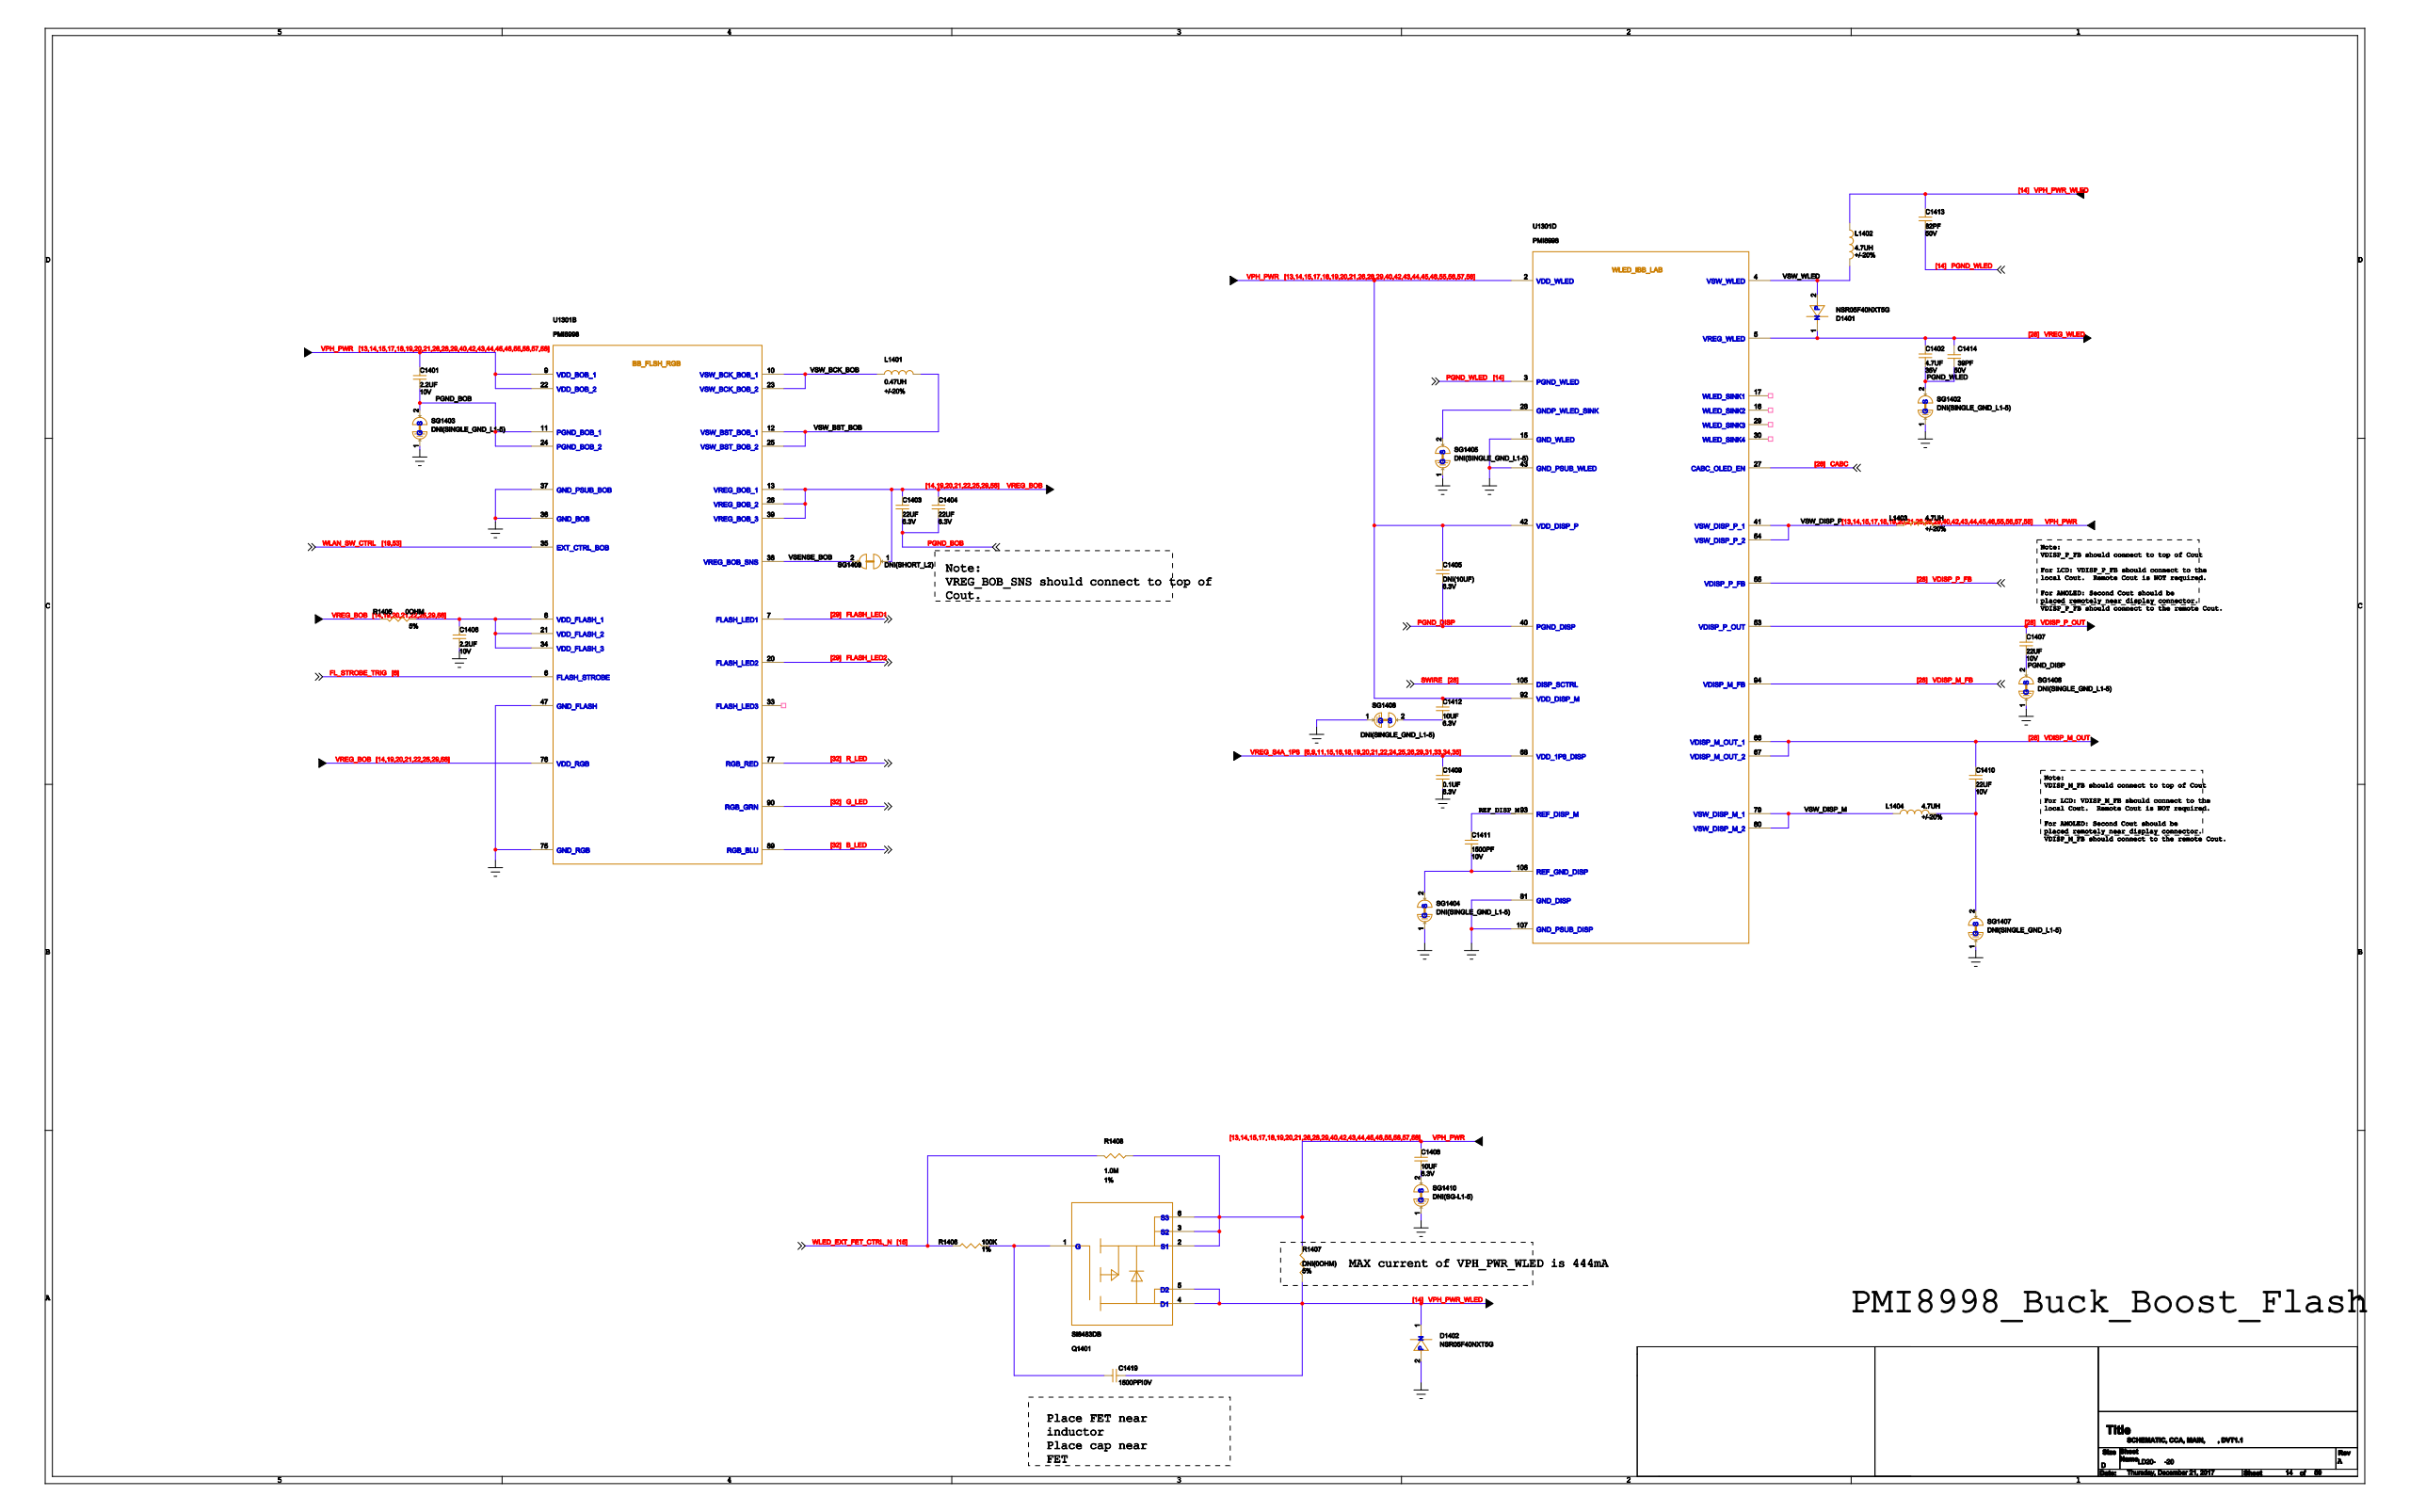Circuit board | Cadence Allegro | 1520 parts | 1149 nets | one sheet of the schematic
Parts on this sheet (reference | value | footprint):
C1401 | 2.2UF | 2P0402R
C1402 | 4.7UF | 2P0603R
C1403 | 22UF | 2P0603R
C1404 | 22UF | 2P0603R
C1405 | DNI(10UF) | 2P0402RV1_DNI
C1406 | 2.2UF | 2P0402R
C1407 | 22UF | 2P0603R
C1408 | 10UF | 2P0402RV1
C1409 | 0.1UF | 2P0201R
C1410 | 22UF | 2P0603R
C1411 | 1500PF | 2P0201R
C1412 | 10UF | 2P0402RV1
C1413 | 82PF | 2P0201R
C1414 | 39PF | 2P0201R
C1419 | 1500PF | 2P0201R
D1401 | NSR05F40NXT5G | 2PSM39X24NV1
D1402 | NSR05F40NXT5G | 2PSM39X24NV1
L1401 | 0.47UH | 2PSM87X71NV2
L1402 | 4.7UH | SL2520
L1403 | 4.7UH | SL2520
L1404 | 4.7UH | SL2520
Q1401 | SI8483DB | 6PGA59X39B197V1
R1405 | 0OHM | 2P0402R
R1406 | 100K | 2P0201R
R1407 | DNI(0OHM) | 2P0402R_DNI
R1408 | 1.0M | 2P0201R
SG1402 | DNI(SINGLE_GND_L1-5) | GND_L1-5
SG1403 | DNI(SINGLE_GND_L1-5) | GND_L1-5
SG1404 | DNI(SINGLE_GND_L1-5) | GND_L1-5
SG1405 | DNI(SINGLE_GND_L1-5) | GND_L1-5
SG1406 | DNI(SINGLE_GND_L1-5) | GND_L1-5
SG1407 | DNI(SINGLE_GND_L1-5) | GND_L1-5
SG1408 | DNI(SINGLE_GND_L1-5) | GND_L1-5
SG1409 | DNI(SHORT_L2) | SHORT_L2_2REC08X12
SG1410 | DNI(SG-L1-5) | SINGLE-GND_L1-5
U1301 | PMI8998 | 182PGA229X212B157
Nets of these parts (net: part-pin ...):
GND: C1406-2 C1409-2 D1402-2 SG1402-1 SG1403-1 SG1404-1 SG1405-1 SG1406-1 SG1407-1 SG1408-1 SG1410-1 U1301-15 U1301-18 U1301-31 U1301-36 U1301-37 U1301-43 U1301-47 U1301-59 U1301-75 U1301-81 U1301-107
VREG_BOB: C1403-1 C1404-1 R1405-1 SG1409-1 U1301-13 U1301-26 U1301-39 U1301-76
VREG_S4A_1P8: C1409-1 U1301-68
FLASH_LED2: U1301-20
FLASH_LED1: U1301-7
PGND_WLED: C1402-2 C1413-2 C1414-1 SG1402-2 U1301-3
PGND_BOB: C1401-2 C1403-2 C1404-2 SG1403-2 U1301-11 U1301-24
N34044332: C1411-2 SG1404-2 U1301-106
N35146226: SG1405-2 U1301-28
PGND_DISP: C1405-2 C1407-2 SG1406-2 U1301-40
N34045940: C1410-2 L1404-2 SG1407-2
N35146965: C1412-2 SG1408-2
VPH_PWR: C1401-1 C1405-1 C1408-1 C1412-1 L1403-2 Q1401-2 Q1401-3 Q1401-6 R1407-1 R1408-2 U1301-2 U1301-9 U1301-22 U1301-42 U1301-92
VSENSE_BOB: SG1409-2 U1301-38
VDISP_P_FB: U1301-55
VDISP_M_FB: U1301-94
N51294727: C1408-2 SG1410-2
VDISP_P_OUT: C1407-1 U1301-53
VREG_WLED: C1402-1 C1414-2 D1401-1 U1301-5
SWIRE: U1301-105
CABC: U1301-27
VPH_PWR_WLED: C1413-1 C1419-2 D1402-1 L1402-1 Q1401-4 Q1401-5 R1407-2
N34042732: C1406-1 R1405-2 U1301-8 U1301-21 U1301-34
VDISP_M_OUT: C1410-1 U1301-66 U1301-67
N43824010: C1419-1 Q1401-1 R1406-1
N34044286: C1411-1 U1301-93
VSW_WLED: D1401-2 L1402-2 U1301-4
B_LED: U1301-89
R_LED: U1301-77
G_LED: U1301-90
VSW_BCK_BOB: L1401-1 U1301-10 U1301-23
VSW_BST_BOB: L1401-2 U1301-12 U1301-25
VSW_DISP_P: L1403-1 U1301-41 U1301-54
VSW_DISP_M: L1404-1 U1301-79 U1301-80
WLED_EXT_FET_CTRL_N: R1406-2 R1408-1 U1301-56
FL_STROBE_TRIG: U1301-6
WLAN_SW_CTRL: U1301-35